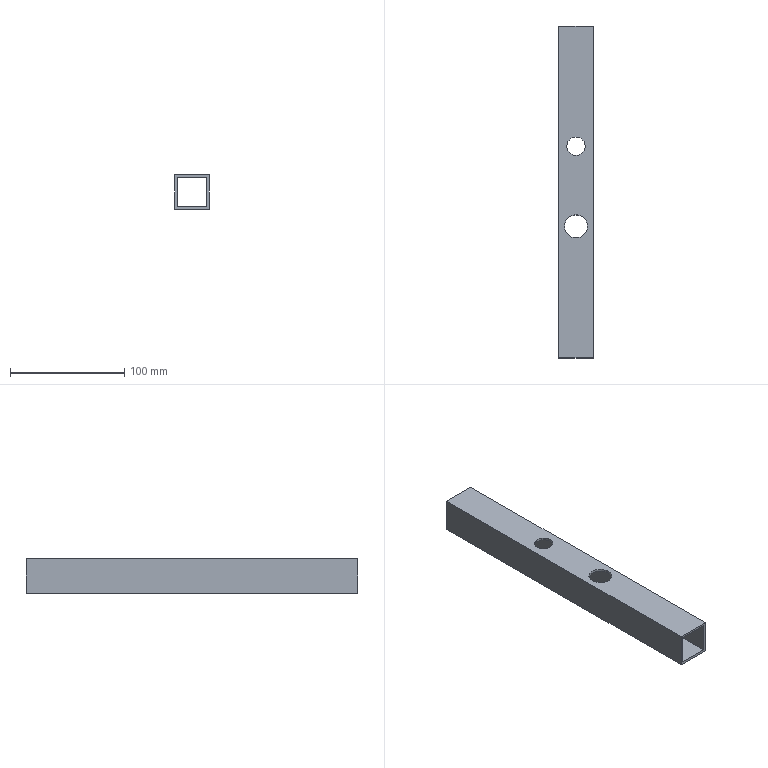Part | NX | features solid 2 | 1 solid | 14 faces | box 30 x 290 x 30 mm | volume 62899 mm3 | plane 10 | cylinder 4 | commonest cylinder face diameters 16 x2 20 x2
STEP:
#1=CARTESIAN_POINT('',(335.,-80.,-10.));
#2=VERTEX_POINT('',#1);
#3=CARTESIAN_POINT('',(325.,-80.,-10.));
#4=DIRECTION('',(0.,0.,1.));
#5=DIRECTION('',(1.,0.,0.));
#6=AXIS2_PLACEMENT_3D('',#3,#4,#5);
#7=CIRCLE('',#6,10.);
#8=EDGE_CURVE('',#2,#2,#7,.T.);
#9=ORIENTED_EDGE('',*,*,#8,.T.);
#10=EDGE_LOOP('',(#9));
#11=FACE_BOUND('',#10,.T.);
#12=CARTESIAN_POINT('',(315.,-80.,-12.));
#13=VERTEX_POINT('',#12);
#14=CARTESIAN_POINT('',(325.,-80.,-12.));
#15=DIRECTION('',(0.,0.,-1.));
#16=DIRECTION('',(-1.,0.,0.));
#17=AXIS2_PLACEMENT_3D('',#14,#15,#16);
#18=CIRCLE('',#17,10.);
#19=EDGE_CURVE('',#13,#13,#18,.F.);
#20=ORIENTED_EDGE('',*,*,#19,.F.);
#21=EDGE_LOOP('',(#20));
#22=FACE_BOUND('',#21,.T.);
#23=CARTESIAN_POINT('',(325.,-80.,18.));
#24=DIRECTION('',(0.,0.,-1.));
#25=DIRECTION('',(-1.,0.,0.));
#26=AXIS2_PLACEMENT_3D('',#23,#24,#25);
#27=CYLINDRICAL_SURFACE('',#26,10.);
#28=ADVANCED_FACE('',(#11,#22),#27,.F.);
#29=CARTESIAN_POINT('',(333.,-10.,-10.));
#30=VERTEX_POINT('',#29);
#31=CARTESIAN_POINT('',(325.,-10.,-10.));
#32=DIRECTION('',(0.,0.,1.));
#33=DIRECTION('',(1.,0.,0.));
#34=AXIS2_PLACEMENT_3D('',#31,#32,#33);
#35=CIRCLE('',#34,8.);
#36=EDGE_CURVE('',#30,#30,#35,.T.);
#37=ORIENTED_EDGE('',*,*,#36,.T.);
#38=EDGE_LOOP('',(#37));
#39=FACE_BOUND('',#38,.T.);
#40=CARTESIAN_POINT('',(317.,-10.,-12.));
#41=VERTEX_POINT('',#40);
#42=CARTESIAN_POINT('',(325.,-10.,-12.));
#43=DIRECTION('',(0.,0.,-1.));
#44=DIRECTION('',(-1.,0.,0.));
#45=AXIS2_PLACEMENT_3D('',#42,#43,#44);
#46=CIRCLE('',#45,8.);
#47=EDGE_CURVE('',#41,#41,#46,.F.);
#48=ORIENTED_EDGE('',*,*,#47,.F.);
#49=EDGE_LOOP('',(#48));
#50=FACE_BOUND('',#49,.T.);
#51=CARTESIAN_POINT('',(325.,-10.,-5.));
#52=DIRECTION('',(0.,0.,-1.));
#53=DIRECTION('',(-1.,0.,0.));
#54=AXIS2_PLACEMENT_3D('',#51,#52,#53);
#55=CYLINDRICAL_SURFACE('',#54,8.);
#56=ADVANCED_FACE('',(#39,#50),#55,.F.);
#57=ORIENTED_EDGE('',*,*,#8,.F.);
#58=EDGE_LOOP('',(#57));
#59=FACE_BOUND('',#58,.T.);
#60=CARTESIAN_POINT('',(310.,-195.,-10.));
#61=VERTEX_POINT('',#60);
#62=CARTESIAN_POINT('',(340.,-195.,-10.));
#63=VERTEX_POINT('',#62);
#64=CARTESIAN_POINT('',(309.,-195.,-10.));
#65=DIRECTION('',(1.,0.,0.));
#66=VECTOR('',#65,1000.);
#67=LINE('',#64,#66);
#68=EDGE_CURVE('',#61,#63,#67,.T.);
#69=ORIENTED_EDGE('',*,*,#68,.T.);
#70=CARTESIAN_POINT('',(340.,95.,-10.));
#71=VERTEX_POINT('',#70);
#72=CARTESIAN_POINT('',(340.,-30.,-10.));
#73=DIRECTION('',(0.,1.,0.));
#74=VECTOR('',#73,1000.);
#75=LINE('',#72,#74);
#76=EDGE_CURVE('',#71,#63,#75,.F.);
#77=ORIENTED_EDGE('',*,*,#76,.F.);
#78=CARTESIAN_POINT('',(310.,95.,-10.));
#79=VERTEX_POINT('',#78);
#80=CARTESIAN_POINT('',(309.,95.,-10.));
#81=DIRECTION('',(-1.,0.,0.));
#82=VECTOR('',#81,1000.);
#83=LINE('',#80,#82);
#84=EDGE_CURVE('',#79,#71,#83,.F.);
#85=ORIENTED_EDGE('',*,*,#84,.F.);
#86=CARTESIAN_POINT('',(310.,-30.,-10.));
#87=DIRECTION('',(0.,-1.,0.));
#88=VECTOR('',#87,1000.);
#89=LINE('',#86,#88);
#90=EDGE_CURVE('',#79,#61,#89,.T.);
#91=ORIENTED_EDGE('',*,*,#90,.T.);
#92=EDGE_LOOP('',(#69,#77,#85,#91));
#93=FACE_BOUND('',#92,.T.);
#94=ORIENTED_EDGE('',*,*,#36,.F.);
#95=EDGE_LOOP('',(#94));
#96=FACE_BOUND('',#95,.T.);
#97=CARTESIAN_POINT('',(309.,-30.,-10.));
#98=DIRECTION('',(0.,0.,1.));
#99=DIRECTION('',(1.,0.,0.));
#100=AXIS2_PLACEMENT_3D('',#97,#98,#99);
#101=PLANE('',#100);
#102=ADVANCED_FACE('',(#59,#93,#96),#101,.T.);
#103=CARTESIAN_POINT('',(335.,-80.,-40.));
#104=VERTEX_POINT('',#103);
#105=CARTESIAN_POINT('',(325.,-80.,-40.));
#106=DIRECTION('',(0.,0.,1.));
#107=DIRECTION('',(1.,0.,0.));
#108=AXIS2_PLACEMENT_3D('',#105,#106,#107);
#109=CIRCLE('',#108,10.);
#110=EDGE_CURVE('',#104,#104,#109,.F.);
#111=ORIENTED_EDGE('',*,*,#110,.F.);
#112=EDGE_LOOP('',(#111));
#113=FACE_BOUND('',#112,.T.);
#114=CARTESIAN_POINT('',(340.,95.,-40.));
#115=VERTEX_POINT('',#114);
#116=CARTESIAN_POINT('',(340.,-195.,-40.));
#117=VERTEX_POINT('',#116);
#118=CARTESIAN_POINT('',(340.,-30.,-40.));
#119=DIRECTION('',(0.,1.,0.));
#120=VECTOR('',#119,1000.);
#121=LINE('',#118,#120);
#122=EDGE_CURVE('',#115,#117,#121,.F.);
#123=ORIENTED_EDGE('',*,*,#122,.T.);
#124=CARTESIAN_POINT('',(310.,-195.,-40.));
#125=VERTEX_POINT('',#124);
#126=CARTESIAN_POINT('',(309.,-195.,-40.));
#127=DIRECTION('',(1.,0.,0.));
#128=VECTOR('',#127,1000.);
#129=LINE('',#126,#128);
#130=EDGE_CURVE('',#125,#117,#129,.T.);
#131=ORIENTED_EDGE('',*,*,#130,.F.);
#132=CARTESIAN_POINT('',(310.,95.,-40.));
#133=VERTEX_POINT('',#132);
#134=CARTESIAN_POINT('',(310.,-30.,-40.));
#135=DIRECTION('',(0.,-1.,0.));
#136=VECTOR('',#135,1000.);
#137=LINE('',#134,#136);
#138=EDGE_CURVE('',#133,#125,#137,.T.);
#139=ORIENTED_EDGE('',*,*,#138,.F.);
#140=CARTESIAN_POINT('',(309.,95.,-40.));
#141=DIRECTION('',(-1.,0.,0.));
#142=VECTOR('',#141,1000.);
#143=LINE('',#140,#142);
#144=EDGE_CURVE('',#133,#115,#143,.F.);
#145=ORIENTED_EDGE('',*,*,#144,.T.);
#146=EDGE_LOOP('',(#123,#131,#139,#145));
#147=FACE_BOUND('',#146,.T.);
#148=CARTESIAN_POINT('',(333.,-10.,-40.));
#149=VERTEX_POINT('',#148);
#150=CARTESIAN_POINT('',(325.,-10.,-40.));
#151=DIRECTION('',(0.,0.,1.));
#152=DIRECTION('',(1.,0.,0.));
#153=AXIS2_PLACEMENT_3D('',#150,#151,#152);
#154=CIRCLE('',#153,8.);
#155=EDGE_CURVE('',#149,#149,#154,.F.);
#156=ORIENTED_EDGE('',*,*,#155,.F.);
#157=EDGE_LOOP('',(#156));
#158=FACE_BOUND('',#157,.T.);
#159=CARTESIAN_POINT('',(309.,-30.,-40.));
#160=DIRECTION('',(0.,0.,1.));
#161=DIRECTION('',(1.,0.,0.));
#162=AXIS2_PLACEMENT_3D('',#159,#160,#161);
#163=PLANE('',#162);
#164=ADVANCED_FACE('',(#113,#147,#158),#163,.F.);
#165=CARTESIAN_POINT('',(338.,95.,-38.));
#166=VERTEX_POINT('',#165);
#167=CARTESIAN_POINT('',(312.,95.,-38.));
#168=VERTEX_POINT('',#167);
#169=CARTESIAN_POINT('',(309.,95.,-38.));
#170=DIRECTION('',(1.,0.,0.));
#171=VECTOR('',#170,1000.);
#172=LINE('',#169,#171);
#173=EDGE_CURVE('',#166,#168,#172,.F.);
#174=ORIENTED_EDGE('',*,*,#173,.F.);
#175=CARTESIAN_POINT('',(338.,95.,-12.));
#176=VERTEX_POINT('',#175);
#177=CARTESIAN_POINT('',(338.,95.,-35.));
#178=DIRECTION('',(0.,0.,-1.));
#179=VECTOR('',#178,1000.);
#180=LINE('',#177,#179);
#181=EDGE_CURVE('',#166,#176,#180,.F.);
#182=ORIENTED_EDGE('',*,*,#181,.T.);
#183=CARTESIAN_POINT('',(312.,95.,-12.));
#184=VERTEX_POINT('',#183);
#185=CARTESIAN_POINT('',(309.,95.,-12.));
#186=DIRECTION('',(1.,0.,0.));
#187=VECTOR('',#186,1000.);
#188=LINE('',#185,#187);
#189=EDGE_CURVE('',#176,#184,#188,.F.);
#190=ORIENTED_EDGE('',*,*,#189,.T.);
#191=CARTESIAN_POINT('',(312.,95.,-35.));
#192=DIRECTION('',(0.,0.,-1.));
#193=VECTOR('',#192,1000.);
#194=LINE('',#191,#193);
#195=EDGE_CURVE('',#168,#184,#194,.F.);
#196=ORIENTED_EDGE('',*,*,#195,.F.);
#197=EDGE_LOOP('',(#174,#182,#190,#196));
#198=FACE_BOUND('',#197,.T.);
#199=CARTESIAN_POINT('',(310.,95.,-35.));
#200=DIRECTION('',(0.,0.,1.));
#201=VECTOR('',#200,1000.);
#202=LINE('',#199,#201);
#203=EDGE_CURVE('',#79,#133,#202,.F.);
#204=ORIENTED_EDGE('',*,*,#203,.F.);
#205=ORIENTED_EDGE('',*,*,#84,.T.);
#206=CARTESIAN_POINT('',(340.,95.,-35.));
#207=DIRECTION('',(0.,0.,-1.));
#208=VECTOR('',#207,1000.);
#209=LINE('',#206,#208);
#210=EDGE_CURVE('',#71,#115,#209,.T.);
#211=ORIENTED_EDGE('',*,*,#210,.T.);
#212=ORIENTED_EDGE('',*,*,#144,.F.);
#213=EDGE_LOOP('',(#204,#205,#211,#212));
#214=FACE_BOUND('',#213,.T.);
#215=CARTESIAN_POINT('',(309.,95.,-35.));
#216=DIRECTION('',(0.,1.,0.));
#217=DIRECTION('',(1.,0.,0.));
#218=AXIS2_PLACEMENT_3D('',#215,#216,#217);
#219=PLANE('',#218);
#220=ADVANCED_FACE('',(#198,#214),#219,.T.);
#221=ORIENTED_EDGE('',*,*,#210,.F.);
#222=ORIENTED_EDGE('',*,*,#76,.T.);
#223=CARTESIAN_POINT('',(340.,-195.,-35.));
#224=DIRECTION('',(0.,0.,1.));
#225=VECTOR('',#224,1000.);
#226=LINE('',#223,#225);
#227=EDGE_CURVE('',#63,#117,#226,.F.);
#228=ORIENTED_EDGE('',*,*,#227,.T.);
#229=ORIENTED_EDGE('',*,*,#122,.F.);
#230=EDGE_LOOP('',(#221,#222,#228,#229));
#231=FACE_BOUND('',#230,.T.);
#232=CARTESIAN_POINT('',(340.,-30.,-35.));
#233=DIRECTION('',(1.,0.,0.));
#234=DIRECTION('',(0.,-1.,0.));
#235=AXIS2_PLACEMENT_3D('',#232,#233,#234);
#236=PLANE('',#235);
#237=ADVANCED_FACE('',(#231),#236,.T.);
#238=CARTESIAN_POINT('',(312.,-195.,-12.));
#239=VERTEX_POINT('',#238);
#240=CARTESIAN_POINT('',(338.,-195.,-12.));
#241=VERTEX_POINT('',#240);
#242=CARTESIAN_POINT('',(309.,-195.,-12.));
#243=DIRECTION('',(1.,0.,0.));
#244=VECTOR('',#243,1000.);
#245=LINE('',#242,#244);
#246=EDGE_CURVE('',#239,#241,#245,.T.);
#247=ORIENTED_EDGE('',*,*,#246,.T.);
#248=CARTESIAN_POINT('',(338.,-195.,-38.));
#249=VERTEX_POINT('',#248);
#250=CARTESIAN_POINT('',(338.,-195.,-35.));
#251=DIRECTION('',(0.,0.,-1.));
#252=VECTOR('',#251,1000.);
#253=LINE('',#250,#252);
#254=EDGE_CURVE('',#241,#249,#253,.T.);
#255=ORIENTED_EDGE('',*,*,#254,.T.);
#256=CARTESIAN_POINT('',(312.,-195.,-38.));
#257=VERTEX_POINT('',#256);
#258=CARTESIAN_POINT('',(309.,-195.,-38.));
#259=DIRECTION('',(1.,0.,0.));
#260=VECTOR('',#259,1000.);
#261=LINE('',#258,#260);
#262=EDGE_CURVE('',#257,#249,#261,.T.);
#263=ORIENTED_EDGE('',*,*,#262,.F.);
#264=CARTESIAN_POINT('',(312.,-195.,-35.));
#265=DIRECTION('',(0.,0.,-1.));
#266=VECTOR('',#265,1000.);
#267=LINE('',#264,#266);
#268=EDGE_CURVE('',#239,#257,#267,.T.);
#269=ORIENTED_EDGE('',*,*,#268,.F.);
#270=EDGE_LOOP('',(#247,#255,#263,#269));
#271=FACE_BOUND('',#270,.T.);
#272=ORIENTED_EDGE('',*,*,#227,.F.);
#273=ORIENTED_EDGE('',*,*,#68,.F.);
#274=CARTESIAN_POINT('',(310.,-195.,-35.));
#275=DIRECTION('',(0.,0.,-1.));
#276=VECTOR('',#275,1000.);
#277=LINE('',#274,#276);
#278=EDGE_CURVE('',#61,#125,#277,.T.);
#279=ORIENTED_EDGE('',*,*,#278,.T.);
#280=ORIENTED_EDGE('',*,*,#130,.T.);
#281=EDGE_LOOP('',(#272,#273,#279,#280));
#282=FACE_BOUND('',#281,.T.);
#283=CARTESIAN_POINT('',(309.,-195.,-35.));
#284=DIRECTION('',(0.,1.,0.));
#285=DIRECTION('',(1.,0.,0.));
#286=AXIS2_PLACEMENT_3D('',#283,#284,#285);
#287=PLANE('',#286);
#288=ADVANCED_FACE('',(#271,#282),#287,.F.);
#289=ORIENTED_EDGE('',*,*,#90,.F.);
#290=ORIENTED_EDGE('',*,*,#203,.T.);
#291=ORIENTED_EDGE('',*,*,#138,.T.);
#292=ORIENTED_EDGE('',*,*,#278,.F.);
#293=EDGE_LOOP('',(#289,#290,#291,#292));
#294=FACE_BOUND('',#293,.T.);
#295=CARTESIAN_POINT('',(310.,-30.,-35.));
#296=DIRECTION('',(1.,0.,0.));
#297=DIRECTION('',(0.,-1.,0.));
#298=AXIS2_PLACEMENT_3D('',#295,#296,#297);
#299=PLANE('',#298);
#300=ADVANCED_FACE('',(#294),#299,.F.);
#301=CARTESIAN_POINT('',(315.,-80.,-38.));
#302=VERTEX_POINT('',#301);
#303=CARTESIAN_POINT('',(325.,-80.,-38.));
#304=DIRECTION('',(0.,0.,-1.));
#305=DIRECTION('',(-1.,0.,0.));
#306=AXIS2_PLACEMENT_3D('',#303,#304,#305);
#307=CIRCLE('',#306,10.);
#308=EDGE_CURVE('',#302,#302,#307,.F.);
#309=ORIENTED_EDGE('',*,*,#308,.T.);
#310=EDGE_LOOP('',(#309));
#311=FACE_BOUND('',#310,.T.);
#312=ORIENTED_EDGE('',*,*,#110,.T.);
#313=EDGE_LOOP('',(#312));
#314=FACE_BOUND('',#313,.T.);
#315=CARTESIAN_POINT('',(325.,-80.,18.));
#316=DIRECTION('',(0.,0.,-1.));
#317=DIRECTION('',(-1.,0.,0.));
#318=AXIS2_PLACEMENT_3D('',#315,#316,#317);
#319=CYLINDRICAL_SURFACE('',#318,10.);
#320=ADVANCED_FACE('',(#311,#314),#319,.F.);
#321=CARTESIAN_POINT('',(317.,-10.,-38.));
#322=VERTEX_POINT('',#321);
#323=CARTESIAN_POINT('',(325.,-10.,-38.));
#324=DIRECTION('',(0.,0.,-1.));
#325=DIRECTION('',(-1.,0.,0.));
#326=AXIS2_PLACEMENT_3D('',#323,#324,#325);
#327=CIRCLE('',#326,8.);
#328=EDGE_CURVE('',#322,#322,#327,.F.);
#329=ORIENTED_EDGE('',*,*,#328,.T.);
#330=EDGE_LOOP('',(#329));
#331=FACE_BOUND('',#330,.T.);
#332=ORIENTED_EDGE('',*,*,#155,.T.);
#333=EDGE_LOOP('',(#332));
#334=FACE_BOUND('',#333,.T.);
#335=CARTESIAN_POINT('',(325.,-10.,-5.));
#336=DIRECTION('',(0.,0.,-1.));
#337=DIRECTION('',(-1.,0.,0.));
#338=AXIS2_PLACEMENT_3D('',#335,#336,#337);
#339=CYLINDRICAL_SURFACE('',#338,8.);
#340=ADVANCED_FACE('',(#331,#334),#339,.F.);
#341=CARTESIAN_POINT('',(312.,-455.,-38.));
#342=DIRECTION('',(0.,1.,0.));
#343=VECTOR('',#342,1000.);
#344=LINE('',#341,#343);
#345=EDGE_CURVE('',#257,#168,#344,.T.);
#346=ORIENTED_EDGE('',*,*,#345,.T.);
#347=ORIENTED_EDGE('',*,*,#195,.T.);
#348=CARTESIAN_POINT('',(312.,-455.,-12.));
#349=DIRECTION('',(0.,1.,0.));
#350=VECTOR('',#349,1000.);
#351=LINE('',#348,#350);
#352=EDGE_CURVE('',#239,#184,#351,.T.);
#353=ORIENTED_EDGE('',*,*,#352,.F.);
#354=ORIENTED_EDGE('',*,*,#268,.T.);
#355=EDGE_LOOP('',(#346,#347,#353,#354));
#356=FACE_BOUND('',#355,.T.);
#357=CARTESIAN_POINT('',(312.,-455.,-35.));
#358=DIRECTION('',(-1.,0.,0.));
#359=DIRECTION('',(0.,0.,1.));
#360=AXIS2_PLACEMENT_3D('',#357,#358,#359);
#361=PLANE('',#360);
#362=ADVANCED_FACE('',(#356),#361,.F.);
#363=ORIENTED_EDGE('',*,*,#181,.F.);
#364=CARTESIAN_POINT('',(338.,-455.,-38.));
#365=DIRECTION('',(0.,1.,0.));
#366=VECTOR('',#365,1000.);
#367=LINE('',#364,#366);
#368=EDGE_CURVE('',#249,#166,#367,.T.);
#369=ORIENTED_EDGE('',*,*,#368,.F.);
#370=ORIENTED_EDGE('',*,*,#254,.F.);
#371=CARTESIAN_POINT('',(338.,-455.,-12.));
#372=DIRECTION('',(0.,1.,0.));
#373=VECTOR('',#372,1000.);
#374=LINE('',#371,#373);
#375=EDGE_CURVE('',#241,#176,#374,.T.);
#376=ORIENTED_EDGE('',*,*,#375,.T.);
#377=EDGE_LOOP('',(#363,#369,#370,#376));
#378=FACE_BOUND('',#377,.T.);
#379=CARTESIAN_POINT('',(338.,-455.,-35.));
#380=DIRECTION('',(-1.,0.,0.));
#381=DIRECTION('',(0.,0.,1.));
#382=AXIS2_PLACEMENT_3D('',#379,#380,#381);
#383=PLANE('',#382);
#384=ADVANCED_FACE('',(#378),#383,.T.);
#385=ORIENTED_EDGE('',*,*,#308,.F.);
#386=EDGE_LOOP('',(#385));
#387=FACE_BOUND('',#386,.T.);
#388=ORIENTED_EDGE('',*,*,#328,.F.);
#389=EDGE_LOOP('',(#388));
#390=FACE_BOUND('',#389,.T.);
#391=ORIENTED_EDGE('',*,*,#368,.T.);
#392=ORIENTED_EDGE('',*,*,#173,.T.);
#393=ORIENTED_EDGE('',*,*,#345,.F.);
#394=ORIENTED_EDGE('',*,*,#262,.T.);
#395=EDGE_LOOP('',(#391,#392,#393,#394));
#396=FACE_BOUND('',#395,.T.);
#397=CARTESIAN_POINT('',(309.,-455.,-38.));
#398=DIRECTION('',(0.,0.,-1.));
#399=DIRECTION('',(-1.,0.,0.));
#400=AXIS2_PLACEMENT_3D('',#397,#398,#399);
#401=PLANE('',#400);
#402=ADVANCED_FACE('',(#387,#390,#396),#401,.F.);
#403=ORIENTED_EDGE('',*,*,#19,.T.);
#404=EDGE_LOOP('',(#403));
#405=FACE_BOUND('',#404,.T.);
#406=ORIENTED_EDGE('',*,*,#47,.T.);
#407=EDGE_LOOP('',(#406));
#408=FACE_BOUND('',#407,.T.);
#409=ORIENTED_EDGE('',*,*,#189,.F.);
#410=ORIENTED_EDGE('',*,*,#375,.F.);
#411=ORIENTED_EDGE('',*,*,#246,.F.);
#412=ORIENTED_EDGE('',*,*,#352,.T.);
#413=EDGE_LOOP('',(#409,#410,#411,#412));
#414=FACE_BOUND('',#413,.T.);
#415=CARTESIAN_POINT('',(309.,-455.,-12.));
#416=DIRECTION('',(0.,0.,-1.));
#417=DIRECTION('',(-1.,0.,0.));
#418=AXIS2_PLACEMENT_3D('',#415,#416,#417);
#419=PLANE('',#418);
#420=ADVANCED_FACE('',(#405,#408,#414),#419,.T.);
#421=CLOSED_SHELL('',(#28,#56,#102,#164,#220,#237,#288,#300,#320,#340,#362,#384,#402,#420));
#422=MANIFOLD_SOLID_BREP('',#421);
#423=(LENGTH_UNIT()NAMED_UNIT(*)SI_UNIT(.MILLI.,.METRE.));
#424=UNCERTAINTY_MEASURE_WITH_UNIT(LENGTH_MEASURE(0.00001),#423,'','');
#425=(NAMED_UNIT(*)PLANE_ANGLE_UNIT()SI_UNIT($,.RADIAN.));
#426=(NAMED_UNIT(*)SI_UNIT($,.STERADIAN.)SOLID_ANGLE_UNIT());
#427=(GEOMETRIC_REPRESENTATION_CONTEXT(3)GLOBAL_UNCERTAINTY_ASSIGNED_CONTEXT((#424))GLOBAL_UNIT_ASSIGNED_CONTEXT((#423,#425,#426))REPRESENTATION_CONTEXT('',''));
#428=ADVANCED_BREP_SHAPE_REPRESENTATION('',(#422),#427);